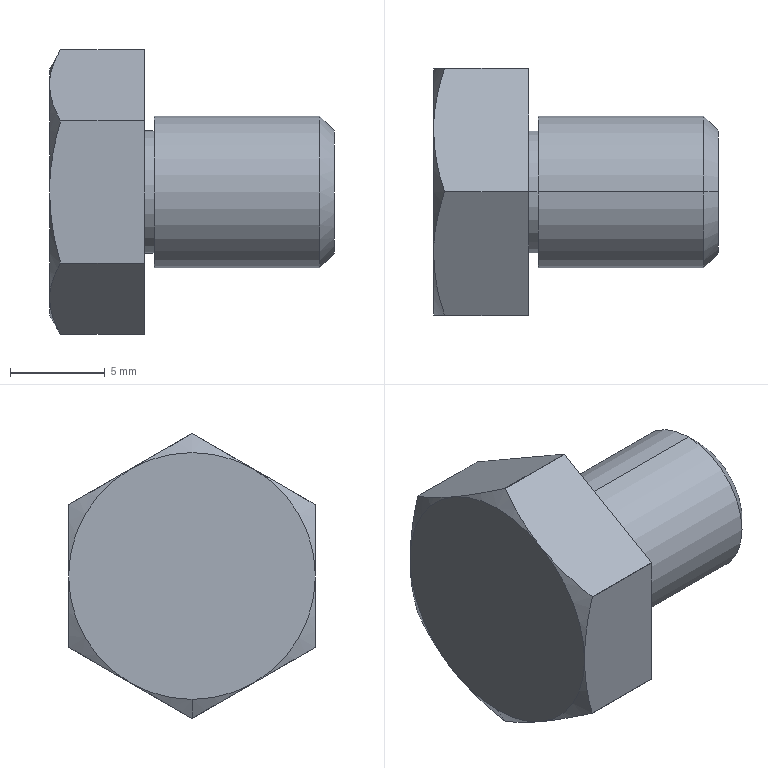Part | STEP file | SSTEH13-4 | 1 solid | 30 faces | box 15 x 13 x 15 mm | volume 1216 mm3 | cylinder 11 | plane 10 | cone 9 | commonest cylinder face diameters 15 x7 6.466 x2 8 x2
STEP:
#1=CARTESIAN_POINT('',(10.,0.,3.233));
#2=VERTEX_POINT('',#1);
#3=CARTESIAN_POINT('',(10.,0.,-3.233));
#4=VERTEX_POINT('',#3);
#5=CARTESIAN_POINT('',(10.,0.,0.));
#6=DIRECTION('',(-1.,0.,0.));
#7=DIRECTION('',(0.,0.,-1.));
#8=AXIS2_PLACEMENT_3D('',#5,#6,#7);
#9=CIRCLE('',#8,3.233);
#10=EDGE_CURVE('',#2,#4,#9,.T.);
#11=ORIENTED_EDGE('',*,*,#10,.T.);
#12=CARTESIAN_POINT('',(9.233,0.,-4.));
#13=VERTEX_POINT('',#12);
#14=CARTESIAN_POINT('',(9.233,0.,-4.));
#15=DIRECTION('',(-0.7071,0.,-0.7071));
#16=VECTOR('',#15,1000.);
#17=LINE('',#14,#16);
#18=EDGE_CURVE('',#4,#13,#17,.T.);
#19=ORIENTED_EDGE('',*,*,#18,.T.);
#20=CARTESIAN_POINT('',(9.233,0.,4.));
#21=VERTEX_POINT('',#20);
#22=CARTESIAN_POINT('',(9.233,0.,0.));
#23=DIRECTION('',(-1.,0.,0.));
#24=DIRECTION('',(0.,0.,-1.));
#25=AXIS2_PLACEMENT_3D('',#22,#23,#24);
#26=CIRCLE('',#25,4.);
#27=EDGE_CURVE('',#21,#13,#26,.T.);
#28=ORIENTED_EDGE('',*,*,#27,.F.);
#29=CARTESIAN_POINT('',(9.233,0.,4.));
#30=DIRECTION('',(-0.7071,0.,0.7071));
#31=VECTOR('',#30,1000.);
#32=LINE('',#29,#31);
#33=EDGE_CURVE('',#2,#21,#32,.T.);
#34=ORIENTED_EDGE('',*,*,#33,.F.);
#35=EDGE_LOOP('',(#11,#19,#28,#34));
#36=FACE_OUTER_BOUND('',#35,.T.);
#37=CARTESIAN_POINT('',(9.233,0.,0.));
#38=DIRECTION('',(-1.,0.,0.));
#39=DIRECTION('',(0.,0.,1.));
#40=AXIS2_PLACEMENT_3D('',#37,#38,#39);
#41=CONICAL_SURFACE('',#40,4.,0.7854);
#42=ADVANCED_FACE('',(#36),#41,.T.);
#43=CARTESIAN_POINT('',(0.5,0.,4.));
#44=VERTEX_POINT('',#43);
#45=CARTESIAN_POINT('',(0.5,0.,-4.));
#46=VERTEX_POINT('',#45);
#47=CARTESIAN_POINT('',(0.5,0.,0.));
#48=DIRECTION('',(-1.,0.,0.));
#49=DIRECTION('',(0.,0.,-1.));
#50=AXIS2_PLACEMENT_3D('',#47,#48,#49);
#51=CIRCLE('',#50,4.);
#52=EDGE_CURVE('',#44,#46,#51,.T.);
#53=ORIENTED_EDGE('',*,*,#52,.F.);
#54=CARTESIAN_POINT('',(10.,0.,4.));
#55=DIRECTION('',(1.,0.,0.));
#56=VECTOR('',#55,1000.);
#57=LINE('',#54,#56);
#58=EDGE_CURVE('',#44,#21,#57,.T.);
#59=ORIENTED_EDGE('',*,*,#58,.T.);
#60=ORIENTED_EDGE('',*,*,#27,.T.);
#61=CARTESIAN_POINT('',(10.,0.,-4.));
#62=DIRECTION('',(1.,0.,0.));
#63=VECTOR('',#62,1000.);
#64=LINE('',#61,#63);
#65=EDGE_CURVE('',#46,#13,#64,.T.);
#66=ORIENTED_EDGE('',*,*,#65,.F.);
#67=EDGE_LOOP('',(#53,#59,#60,#66));
#68=FACE_OUTER_BOUND('',#67,.T.);
#69=CARTESIAN_POINT('',(10.,0.,0.));
#70=DIRECTION('',(1.,0.,0.));
#71=DIRECTION('',(0.,0.,-1.));
#72=AXIS2_PLACEMENT_3D('',#69,#70,#71);
#73=CYLINDRICAL_SURFACE('',#72,4.);
#74=ADVANCED_FACE('',(#68),#73,.T.);
#75=CARTESIAN_POINT('',(0.,0.,3.233));
#76=VERTEX_POINT('',#75);
#77=CARTESIAN_POINT('',(0.,0.,-3.233));
#78=VERTEX_POINT('',#77);
#79=CARTESIAN_POINT('',(0.,0.,0.));
#80=DIRECTION('',(-1.,0.,0.));
#81=DIRECTION('',(0.,0.,-1.));
#82=AXIS2_PLACEMENT_3D('',#79,#80,#81);
#83=CIRCLE('',#82,3.233);
#84=EDGE_CURVE('',#76,#78,#83,.T.);
#85=ORIENTED_EDGE('',*,*,#84,.F.);
#86=CARTESIAN_POINT('',(0.5,0.,3.233));
#87=VERTEX_POINT('',#86);
#88=CARTESIAN_POINT('',(10.,0.,3.233));
#89=DIRECTION('',(1.,0.,0.));
#90=VECTOR('',#89,1000.);
#91=LINE('',#88,#90);
#92=EDGE_CURVE('',#76,#87,#91,.T.);
#93=ORIENTED_EDGE('',*,*,#92,.T.);
#94=CARTESIAN_POINT('',(0.5,0.,-3.233));
#95=VERTEX_POINT('',#94);
#96=CARTESIAN_POINT('',(0.5,0.,0.));
#97=DIRECTION('',(-1.,0.,0.));
#98=DIRECTION('',(0.,0.,-1.));
#99=AXIS2_PLACEMENT_3D('',#96,#97,#98);
#100=CIRCLE('',#99,3.233);
#101=EDGE_CURVE('',#87,#95,#100,.T.);
#102=ORIENTED_EDGE('',*,*,#101,.T.);
#103=CARTESIAN_POINT('',(10.,0.,-3.233));
#104=DIRECTION('',(1.,0.,0.));
#105=VECTOR('',#104,1000.);
#106=LINE('',#103,#105);
#107=EDGE_CURVE('',#78,#95,#106,.T.);
#108=ORIENTED_EDGE('',*,*,#107,.F.);
#109=EDGE_LOOP('',(#85,#93,#102,#108));
#110=FACE_OUTER_BOUND('',#109,.T.);
#111=CARTESIAN_POINT('',(10.,0.,0.));
#112=DIRECTION('',(1.,0.,0.));
#113=DIRECTION('',(0.,0.,-1.));
#114=AXIS2_PLACEMENT_3D('',#111,#112,#113);
#115=CYLINDRICAL_SURFACE('',#114,3.233);
#116=ADVANCED_FACE('',(#110),#115,.T.);
#117=CARTESIAN_POINT('',(-4.423,0.,-7.5));
#118=VERTEX_POINT('',#117);
#119=CARTESIAN_POINT('',(-4.423,-0.00963,-7.5));
#120=VERTEX_POINT('',#119);
#121=CARTESIAN_POINT('',(-4.423,0.,0.));
#122=DIRECTION('',(-1.,0.,0.));
#123=DIRECTION('',(0.,0.,-1.));
#124=AXIS2_PLACEMENT_3D('',#121,#122,#123);
#125=CIRCLE('',#124,7.5);
#126=EDGE_CURVE('',#118,#120,#125,.T.);
#127=ORIENTED_EDGE('',*,*,#126,.F.);
#128=CARTESIAN_POINT('',(0.,0.,-7.5));
#129=VERTEX_POINT('',#128);
#130=CARTESIAN_POINT('',(10.,0.,-7.5));
#131=DIRECTION('',(1.,0.,0.));
#132=VECTOR('',#131,1000.);
#133=LINE('',#130,#132);
#134=EDGE_CURVE('',#118,#129,#133,.T.);
#135=ORIENTED_EDGE('',*,*,#134,.T.);
#136=CARTESIAN_POINT('',(0.,-0.00963,-7.5));
#137=VERTEX_POINT('',#136);
#138=CARTESIAN_POINT('',(0.,0.,0.));
#139=DIRECTION('',(-1.,0.,0.));
#140=DIRECTION('',(0.,0.,-1.));
#141=AXIS2_PLACEMENT_3D('',#138,#139,#140);
#142=CIRCLE('',#141,7.5);
#143=EDGE_CURVE('',#129,#137,#142,.T.);
#144=ORIENTED_EDGE('',*,*,#143,.T.);
#145=CARTESIAN_POINT('',(10.,-0.00963,-7.5));
#146=DIRECTION('',(-1.,0.,0.));
#147=VECTOR('',#146,1000.);
#148=LINE('',#145,#147);
#149=EDGE_CURVE('',#137,#120,#148,.T.);
#150=ORIENTED_EDGE('',*,*,#149,.T.);
#151=EDGE_LOOP('',(#127,#135,#144,#150));
#152=FACE_OUTER_BOUND('',#151,.T.);
#153=CARTESIAN_POINT('',(10.,0.,0.));
#154=DIRECTION('',(1.,0.,0.));
#155=DIRECTION('',(0.,0.,-1.));
#156=AXIS2_PLACEMENT_3D('',#153,#154,#155);
#157=CYLINDRICAL_SURFACE('',#156,7.5);
#158=ADVANCED_FACE('',(#152),#157,.T.);
#159=CARTESIAN_POINT('',(-5.,0.,-6.5));
#160=VERTEX_POINT('',#159);
#161=CARTESIAN_POINT('',(-5.,-3.25,-5.629));
#162=VERTEX_POINT('',#161);
#163=CARTESIAN_POINT('',(-5.,0.,0.));
#164=DIRECTION('',(-1.,0.,0.));
#165=DIRECTION('',(0.,0.,-1.));
#166=AXIS2_PLACEMENT_3D('',#163,#164,#165);
#167=CIRCLE('',#166,6.5);
#168=EDGE_CURVE('',#160,#162,#167,.T.);
#169=ORIENTED_EDGE('',*,*,#168,.F.);
#170=CARTESIAN_POINT('',(-5.,0.,-6.5));
#171=DIRECTION('',(0.5,0.,-0.866));
#172=VECTOR('',#171,1000.);
#173=LINE('',#170,#172);
#174=EDGE_CURVE('',#160,#118,#173,.T.);
#175=ORIENTED_EDGE('',*,*,#174,.T.);
#176=ORIENTED_EDGE('',*,*,#126,.T.);
#177=CARTESIAN_POINT('',(-4.423,-0.00963,-7.5));
#178=CARTESIAN_POINT('',(-4.599,-0.5398,-7.194));
#179=CARTESIAN_POINT('',(-4.744,-1.074,-6.886));
#180=CARTESIAN_POINT('',(-4.945,-2.153,-6.263));
#181=CARTESIAN_POINT('',(-5.,-2.698,-5.948));
#182=CARTESIAN_POINT('',(-5.,-3.25,-5.629));
#183=B_SPLINE_CURVE_WITH_KNOTS('',3,(#177,#178,#179,#180,#181,#182),.UNSPECIFIED.,.F.,.F.,(4,2,4),(0.000000425,0.001893,0.003786),.UNSPECIFIED.);
#184=EDGE_CURVE('',#120,#162,#183,.T.);
#185=ORIENTED_EDGE('',*,*,#184,.T.);
#186=EDGE_LOOP('',(#169,#175,#176,#185));
#187=FACE_OUTER_BOUND('',#186,.T.);
#188=CARTESIAN_POINT('',(-5.,0.,0.));
#189=DIRECTION('',(1.,0.,0.));
#190=DIRECTION('',(0.,0.,-1.));
#191=AXIS2_PLACEMENT_3D('',#188,#189,#190);
#192=CONICAL_SURFACE('',#191,6.5,1.047);
#193=ADVANCED_FACE('',(#187),#192,.T.);
#194=CARTESIAN_POINT('',(-4.423,6.5,3.742));
#195=VERTEX_POINT('',#194);
#196=CARTESIAN_POINT('',(-5.,6.5,0.));
#197=VERTEX_POINT('',#196);
#198=CARTESIAN_POINT('',(-4.423,6.5,3.742));
#199=CARTESIAN_POINT('',(-4.774,6.5,2.523));
#200=CARTESIAN_POINT('',(-5.,6.5,1.281));
#201=CARTESIAN_POINT('',(-5.,6.5,0.));
#202=B_SPLINE_CURVE_WITH_KNOTS('',3,(#198,#199,#200,#201),.UNSPECIFIED.,.F.,.F.,(4,4),(0.008188,0.01199),.UNSPECIFIED.);
#203=EDGE_CURVE('',#195,#197,#202,.T.);
#204=ORIENTED_EDGE('',*,*,#203,.T.);
#205=CARTESIAN_POINT('',(-5.,3.25,5.629));
#206=VERTEX_POINT('',#205);
#207=CARTESIAN_POINT('',(-5.,0.,0.));
#208=DIRECTION('',(-1.,0.,0.));
#209=DIRECTION('',(0.,0.,-1.));
#210=AXIS2_PLACEMENT_3D('',#207,#208,#209);
#211=CIRCLE('',#210,6.5);
#212=EDGE_CURVE('',#206,#197,#211,.T.);
#213=ORIENTED_EDGE('',*,*,#212,.F.);
#214=CARTESIAN_POINT('',(-4.423,6.49,3.758));
#215=VERTEX_POINT('',#214);
#216=CARTESIAN_POINT('',(-5.,3.25,5.629));
#217=CARTESIAN_POINT('',(-5.,3.525,5.47));
#218=CARTESIAN_POINT('',(-4.986,3.801,5.311));
#219=CARTESIAN_POINT('',(-4.934,4.348,4.995));
#220=CARTESIAN_POINT('',(-4.894,4.619,4.839));
#221=CARTESIAN_POINT('',(-4.744,5.428,4.371));
#222=CARTESIAN_POINT('',(-4.599,5.962,4.064));
#223=CARTESIAN_POINT('',(-4.423,6.49,3.758));
#224=B_SPLINE_CURVE_WITH_KNOTS('',3,(#216,#217,#218,#219,#220,#221,#222,#223),.UNSPECIFIED.,.F.,.F.,(4,2,2,4),(0.003786,0.004729,0.005672,0.007557),.UNSPECIFIED.);
#225=EDGE_CURVE('',#206,#215,#224,.T.);
#226=ORIENTED_EDGE('',*,*,#225,.T.);
#227=CARTESIAN_POINT('',(-4.423,0.,0.));
#228=DIRECTION('',(-1.,0.,0.));
#229=DIRECTION('',(0.,0.,-1.));
#230=AXIS2_PLACEMENT_3D('',#227,#228,#229);
#231=CIRCLE('',#230,7.5);
#232=EDGE_CURVE('',#215,#195,#231,.T.);
#233=ORIENTED_EDGE('',*,*,#232,.T.);
#234=EDGE_LOOP('',(#204,#213,#226,#233));
#235=FACE_OUTER_BOUND('',#234,.T.);
#236=CARTESIAN_POINT('',(-5.,0.,0.));
#237=DIRECTION('',(1.,0.,0.));
#238=DIRECTION('',(0.,0.,-1.));
#239=AXIS2_PLACEMENT_3D('',#236,#237,#238);
#240=CONICAL_SURFACE('',#239,6.5,1.047);
#241=ADVANCED_FACE('',(#235),#240,.T.);
#242=CARTESIAN_POINT('',(-4.423,6.5,-3.742));
#243=VERTEX_POINT('',#242);
#244=CARTESIAN_POINT('',(-5.,6.5,0.));
#245=CARTESIAN_POINT('',(-5.,6.5,-0.6403));
#246=CARTESIAN_POINT('',(-4.944,6.5,-1.273));
#247=CARTESIAN_POINT('',(-4.743,6.5,-2.518));
#248=CARTESIAN_POINT('',(-4.598,6.5,-3.133));
#249=CARTESIAN_POINT('',(-4.423,6.5,-3.742));
#250=B_SPLINE_CURVE_WITH_KNOTS('',3,(#244,#245,#246,#247,#248,#249),.UNSPECIFIED.,.F.,.F.,(4,2,4),(0.01199,0.0139,0.0158),.UNSPECIFIED.);
#251=EDGE_CURVE('',#197,#243,#250,.T.);
#252=ORIENTED_EDGE('',*,*,#251,.T.);
#253=CARTESIAN_POINT('',(-4.423,6.49,-3.758));
#254=VERTEX_POINT('',#253);
#255=CARTESIAN_POINT('',(-4.423,0.,0.));
#256=DIRECTION('',(-1.,0.,0.));
#257=DIRECTION('',(0.,0.,-1.));
#258=AXIS2_PLACEMENT_3D('',#255,#256,#257);
#259=CIRCLE('',#258,7.5);
#260=EDGE_CURVE('',#243,#254,#259,.T.);
#261=ORIENTED_EDGE('',*,*,#260,.T.);
#262=CARTESIAN_POINT('',(-5.,3.25,-5.629));
#263=VERTEX_POINT('',#262);
#264=CARTESIAN_POINT('',(-4.423,6.49,-3.758));
#265=CARTESIAN_POINT('',(-4.599,5.96,-4.064));
#266=CARTESIAN_POINT('',(-4.744,5.426,-4.373));
#267=CARTESIAN_POINT('',(-4.945,4.347,-4.996));
#268=CARTESIAN_POINT('',(-5.,3.802,-5.31));
#269=CARTESIAN_POINT('',(-5.,3.25,-5.629));
#270=B_SPLINE_CURVE_WITH_KNOTS('',3,(#264,#265,#266,#267,#268,#269),.UNSPECIFIED.,.F.,.F.,(4,2,4),(0.000000716,0.001894,0.003786),.UNSPECIFIED.);
#271=EDGE_CURVE('',#254,#263,#270,.T.);
#272=ORIENTED_EDGE('',*,*,#271,.T.);
#273=CARTESIAN_POINT('',(-5.,0.,0.));
#274=DIRECTION('',(-1.,0.,0.));
#275=DIRECTION('',(0.,0.,-1.));
#276=AXIS2_PLACEMENT_3D('',#273,#274,#275);
#277=CIRCLE('',#276,6.5);
#278=EDGE_CURVE('',#197,#263,#277,.T.);
#279=ORIENTED_EDGE('',*,*,#278,.F.);
#280=EDGE_LOOP('',(#252,#261,#272,#279));
#281=FACE_OUTER_BOUND('',#280,.T.);
#282=CARTESIAN_POINT('',(-5.,0.,0.));
#283=DIRECTION('',(1.,0.,0.));
#284=DIRECTION('',(0.,0.,-1.));
#285=AXIS2_PLACEMENT_3D('',#282,#283,#284);
#286=CONICAL_SURFACE('',#285,6.5,1.047);
#287=ADVANCED_FACE('',(#281),#286,.T.);
#288=ORIENTED_EDGE('',*,*,#174,.F.);
#289=CARTESIAN_POINT('',(-5.,0.,0.));
#290=DIRECTION('',(-1.,0.,0.));
#291=DIRECTION('',(0.,0.,-1.));
#292=AXIS2_PLACEMENT_3D('',#289,#290,#291);
#293=CIRCLE('',#292,6.5);
#294=EDGE_CURVE('',#263,#160,#293,.T.);
#295=ORIENTED_EDGE('',*,*,#294,.F.);
#296=CARTESIAN_POINT('',(-4.423,0.00963,-7.5));
#297=VERTEX_POINT('',#296);
#298=CARTESIAN_POINT('',(-5.,3.25,-5.629));
#299=CARTESIAN_POINT('',(-5.,2.975,-5.788));
#300=CARTESIAN_POINT('',(-4.986,2.699,-5.947));
#301=CARTESIAN_POINT('',(-4.934,2.152,-6.263));
#302=CARTESIAN_POINT('',(-4.894,1.881,-6.42));
#303=CARTESIAN_POINT('',(-4.744,1.072,-6.887));
#304=CARTESIAN_POINT('',(-4.599,0.5384,-7.195));
#305=CARTESIAN_POINT('',(-4.423,0.00963,-7.5));
#306=B_SPLINE_CURVE_WITH_KNOTS('',3,(#298,#299,#300,#301,#302,#303,#304,#305),.UNSPECIFIED.,.F.,.F.,(4,2,2,4),(0.003786,0.004729,0.005672,0.007558),.UNSPECIFIED.);
#307=EDGE_CURVE('',#263,#297,#306,.T.);
#308=ORIENTED_EDGE('',*,*,#307,.T.);
#309=CARTESIAN_POINT('',(-4.423,0.,0.));
#310=DIRECTION('',(-1.,0.,0.));
#311=DIRECTION('',(0.,0.,-1.));
#312=AXIS2_PLACEMENT_3D('',#309,#310,#311);
#313=CIRCLE('',#312,7.5);
#314=EDGE_CURVE('',#297,#118,#313,.T.);
#315=ORIENTED_EDGE('',*,*,#314,.T.);
#316=EDGE_LOOP('',(#288,#295,#308,#315));
#317=FACE_OUTER_BOUND('',#316,.T.);
#318=CARTESIAN_POINT('',(-5.,0.,0.));
#319=DIRECTION('',(1.,0.,0.));
#320=DIRECTION('',(0.,0.,-1.));
#321=AXIS2_PLACEMENT_3D('',#318,#319,#320);
#322=CONICAL_SURFACE('',#321,6.5,1.047);
#323=ADVANCED_FACE('',(#317),#322,.T.);
#324=CARTESIAN_POINT('',(-4.423,-6.49,-3.758));
#325=VERTEX_POINT('',#324);
#326=CARTESIAN_POINT('',(-5.,-3.25,-5.629));
#327=CARTESIAN_POINT('',(-5.,-3.525,-5.47));
#328=CARTESIAN_POINT('',(-4.986,-3.801,-5.311));
#329=CARTESIAN_POINT('',(-4.934,-4.348,-4.995));
#330=CARTESIAN_POINT('',(-4.894,-4.619,-4.839));
#331=CARTESIAN_POINT('',(-4.744,-5.428,-4.371));
#332=CARTESIAN_POINT('',(-4.599,-5.962,-4.064));
#333=CARTESIAN_POINT('',(-4.423,-6.49,-3.758));
#334=B_SPLINE_CURVE_WITH_KNOTS('',3,(#326,#327,#328,#329,#330,#331,#332,#333),.UNSPECIFIED.,.F.,.F.,(4,2,2,4),(0.003786,0.004729,0.005672,0.007557),.UNSPECIFIED.);
#335=EDGE_CURVE('',#162,#325,#334,.T.);
#336=ORIENTED_EDGE('',*,*,#335,.T.);
#337=CARTESIAN_POINT('',(-4.423,-6.5,-3.742));
#338=VERTEX_POINT('',#337);
#339=CARTESIAN_POINT('',(-4.423,0.,0.));
#340=DIRECTION('',(-1.,0.,0.));
#341=DIRECTION('',(0.,0.,-1.));
#342=AXIS2_PLACEMENT_3D('',#339,#340,#341);
#343=CIRCLE('',#342,7.5);
#344=EDGE_CURVE('',#325,#338,#343,.T.);
#345=ORIENTED_EDGE('',*,*,#344,.T.);
#346=CARTESIAN_POINT('',(-5.,-6.5,0.));
#347=VERTEX_POINT('',#346);
#348=CARTESIAN_POINT('',(-4.423,-6.5,-3.742));
#349=CARTESIAN_POINT('',(-4.774,-6.5,-2.523));
#350=CARTESIAN_POINT('',(-5.,-6.5,-1.281));
#351=CARTESIAN_POINT('',(-5.,-6.5,0.));
#352=B_SPLINE_CURVE_WITH_KNOTS('',3,(#348,#349,#350,#351),.UNSPECIFIED.,.F.,.F.,(4,4),(0.008188,0.01199),.UNSPECIFIED.);
#353=EDGE_CURVE('',#338,#347,#352,.T.);
#354=ORIENTED_EDGE('',*,*,#353,.T.);
#355=CARTESIAN_POINT('',(-5.,0.,0.));
#356=DIRECTION('',(-1.,0.,0.));
#357=DIRECTION('',(0.,0.,-1.));
#358=AXIS2_PLACEMENT_3D('',#355,#356,#357);
#359=CIRCLE('',#358,6.5);
#360=EDGE_CURVE('',#162,#347,#359,.T.);
#361=ORIENTED_EDGE('',*,*,#360,.F.);
#362=EDGE_LOOP('',(#336,#345,#354,#361));
#363=FACE_OUTER_BOUND('',#362,.T.);
#364=CARTESIAN_POINT('',(-5.,0.,0.));
#365=DIRECTION('',(1.,0.,0.));
#366=DIRECTION('',(0.,0.,-1.));
#367=AXIS2_PLACEMENT_3D('',#364,#365,#366);
#368=CONICAL_SURFACE('',#367,6.5,1.047);
#369=ADVANCED_FACE('',(#363),#368,.T.);
#370=CARTESIAN_POINT('',(-4.423,-6.5,3.742));
#371=VERTEX_POINT('',#370);
#372=CARTESIAN_POINT('',(-5.,-6.5,0.));
#373=CARTESIAN_POINT('',(-5.,-6.5,0.6403));
#374=CARTESIAN_POINT('',(-4.944,-6.5,1.273));
#375=CARTESIAN_POINT('',(-4.743,-6.5,2.518));
#376=CARTESIAN_POINT('',(-4.598,-6.5,3.133));
#377=CARTESIAN_POINT('',(-4.423,-6.5,3.742));
#378=B_SPLINE_CURVE_WITH_KNOTS('',3,(#372,#373,#374,#375,#376,#377),.UNSPECIFIED.,.F.,.F.,(4,2,4),(0.01199,0.0139,0.0158),.UNSPECIFIED.);
#379=EDGE_CURVE('',#347,#371,#378,.T.);
#380=ORIENTED_EDGE('',*,*,#379,.T.);
#381=CARTESIAN_POINT('',(-4.423,-6.49,3.758));
#382=VERTEX_POINT('',#381);
#383=CARTESIAN_POINT('',(-4.423,0.,0.));
#384=DIRECTION('',(-1.,0.,0.));
#385=DIRECTION('',(0.,0.,-1.));
#386=AXIS2_PLACEMENT_3D('',#383,#384,#385);
#387=CIRCLE('',#386,7.5);
#388=EDGE_CURVE('',#371,#382,#387,.T.);
#389=ORIENTED_EDGE('',*,*,#388,.T.);
#390=CARTESIAN_POINT('',(-5.,-3.25,5.629));
#391=VERTEX_POINT('',#390);
#392=CARTESIAN_POINT('',(-4.423,-6.49,3.758));
#393=CARTESIAN_POINT('',(-4.599,-5.96,4.064));
#394=CARTESIAN_POINT('',(-4.744,-5.426,4.373));
#395=CARTESIAN_POINT('',(-4.945,-4.347,4.996));
#396=CARTESIAN_POINT('',(-5.,-3.802,5.31));
#397=CARTESIAN_POINT('',(-5.,-3.25,5.629));
#398=B_SPLINE_CURVE_WITH_KNOTS('',3,(#392,#393,#394,#395,#396,#397),.UNSPECIFIED.,.F.,.F.,(4,2,4),(0.000000716,0.001894,0.003786),.UNSPECIFIED.);
#399=EDGE_CURVE('',#382,#391,#398,.T.);
#400=ORIENTED_EDGE('',*,*,#399,.T.);
#401=CARTESIAN_POINT('',(-5.,0.,0.));
#402=DIRECTION('',(-1.,0.,0.));
#403=DIRECTION('',(0.,0.,-1.));
#404=AXIS2_PLACEMENT_3D('',#401,#402,#403);
#405=CIRCLE('',#404,6.5);
#406=EDGE_CURVE('',#347,#391,#405,.T.);
#407=ORIENTED_EDGE('',*,*,#406,.F.);
#408=EDGE_LOOP('',(#380,#389,#400,#407));
#409=FACE_OUTER_BOUND('',#408,.T.);
#410=CARTESIAN_POINT('',(-5.,0.,0.));
#411=DIRECTION('',(1.,0.,0.));
#412=DIRECTION('',(0.,0.,-1.));
#413=AXIS2_PLACEMENT_3D('',#410,#411,#412);
#414=CONICAL_SURFACE('',#413,6.5,1.047);
#415=ADVANCED_FACE('',(#409),#414,.T.);
#416=CARTESIAN_POINT('',(-4.423,-0.00963,7.5));
#417=VERTEX_POINT('',#416);
#418=CARTESIAN_POINT('',(-5.,-3.25,5.629));
#419=CARTESIAN_POINT('',(-5.,-2.975,5.788));
#420=CARTESIAN_POINT('',(-4.986,-2.699,5.947));
#421=CARTESIAN_POINT('',(-4.934,-2.152,6.263));
#422=CARTESIAN_POINT('',(-4.894,-1.881,6.42));
#423=CARTESIAN_POINT('',(-4.744,-1.072,6.887));
#424=CARTESIAN_POINT('',(-4.599,-0.5384,7.195));
#425=CARTESIAN_POINT('',(-4.423,-0.00963,7.5));
#426=B_SPLINE_CURVE_WITH_KNOTS('',3,(#418,#419,#420,#421,#422,#423,#424,#425),.UNSPECIFIED.,.F.,.F.,(4,2,2,4),(0.003786,0.004729,0.005672,0.007558),.UNSPECIFIED.);
#427=EDGE_CURVE('',#391,#417,#426,.T.);
#428=ORIENTED_EDGE('',*,*,#427,.T.);
#429=CARTESIAN_POINT('',(-4.423,0.00963,7.5));
#430=VERTEX_POINT('',#429);
#431=CARTESIAN_POINT('',(-4.423,0.,0.));
#432=DIRECTION('',(-1.,0.,0.));
#433=DIRECTION('',(0.,0.,-1.));
#434=AXIS2_PLACEMENT_3D('',#431,#432,#433);
#435=CIRCLE('',#434,7.5);
#436=EDGE_CURVE('',#417,#430,#435,.T.);
#437=ORIENTED_EDGE('',*,*,#436,.T.);
#438=CARTESIAN_POINT('',(-4.423,0.00963,7.5));
#439=CARTESIAN_POINT('',(-4.599,0.5398,7.194));
#440=CARTESIAN_POINT('',(-4.744,1.074,6.886));
#441=CARTESIAN_POINT('',(-4.945,2.153,6.263));
#442=CARTESIAN_POINT('',(-5.,2.698,5.948));
#443=CARTESIAN_POINT('',(-5.,3.25,5.629));
#444=B_SPLINE_CURVE_WITH_KNOTS('',3,(#438,#439,#440,#441,#442,#443),.UNSPECIFIED.,.F.,.F.,(4,2,4),(0.000000425,0.001893,0.003786),.UNSPECIFIED.);
#445=EDGE_CURVE('',#430,#206,#444,.T.);
#446=ORIENTED_EDGE('',*,*,#445,.T.);
#447=CARTESIAN_POINT('',(-5.,0.,0.));
#448=DIRECTION('',(-1.,0.,0.));
#449=DIRECTION('',(0.,0.,-1.));
#450=AXIS2_PLACEMENT_3D('',#447,#448,#449);
#451=CIRCLE('',#450,6.5);
#452=EDGE_CURVE('',#391,#206,#451,.T.);
#453=ORIENTED_EDGE('',*,*,#452,.F.);
#454=EDGE_LOOP('',(#428,#437,#446,#453));
#455=FACE_OUTER_BOUND('',#454,.T.);
#456=CARTESIAN_POINT('',(-5.,0.,0.));
#457=DIRECTION('',(1.,0.,0.));
#458=DIRECTION('',(0.,0.,-1.));
#459=AXIS2_PLACEMENT_3D('',#456,#457,#458);
#460=CONICAL_SURFACE('',#459,6.5,1.047);
#461=ADVANCED_FACE('',(#455),#460,.T.);
#462=CARTESIAN_POINT('',(0.,6.5,-3.742));
#463=VERTEX_POINT('',#462);
#464=CARTESIAN_POINT('',(10.,6.5,-3.742));
#465=DIRECTION('',(1.,0.,0.));
#466=VECTOR('',#465,1000.);
#467=LINE('',#464,#466);
#468=EDGE_CURVE('',#243,#463,#467,.T.);
#469=ORIENTED_EDGE('',*,*,#468,.T.);
#470=CARTESIAN_POINT('',(0.,6.49,-3.758));
#471=VERTEX_POINT('',#470);
#472=CARTESIAN_POINT('',(0.,0.,0.));
#473=DIRECTION('',(-1.,0.,0.));
#474=DIRECTION('',(0.,0.,-1.));
#475=AXIS2_PLACEMENT_3D('',#472,#473,#474);
#476=CIRCLE('',#475,7.5);
#477=EDGE_CURVE('',#463,#471,#476,.T.);
#478=ORIENTED_EDGE('',*,*,#477,.T.);
#479=CARTESIAN_POINT('',(10.,6.49,-3.758));
#480=DIRECTION('',(-1.,0.,0.));
#481=VECTOR('',#480,1000.);
#482=LINE('',#479,#481);
#483=EDGE_CURVE('',#471,#254,#482,.T.);
#484=ORIENTED_EDGE('',*,*,#483,.T.);
#485=ORIENTED_EDGE('',*,*,#260,.F.);
#486=EDGE_LOOP('',(#469,#478,#484,#485));
#487=FACE_OUTER_BOUND('',#486,.T.);
#488=CARTESIAN_POINT('',(10.,0.,0.));
#489=DIRECTION('',(1.,0.,0.));
#490=DIRECTION('',(0.,0.,-1.));
#491=AXIS2_PLACEMENT_3D('',#488,#489,#490);
#492=CYLINDRICAL_SURFACE('',#491,7.5);
#493=ADVANCED_FACE('',(#487),#492,.T.);
#494=CARTESIAN_POINT('',(0.,6.5,3.742));
#495=VERTEX_POINT('',#494);
#496=CARTESIAN_POINT('',(10.,6.5,3.742));
#497=DIRECTION('',(-1.,0.,0.));
#498=VECTOR('',#497,1000.);
#499=LINE('',#496,#498);
#500=EDGE_CURVE('',#495,#195,#499,.T.);
#501=ORIENTED_EDGE('',*,*,#500,.T.);
#502=ORIENTED_EDGE('',*,*,#232,.F.);
#503=CARTESIAN_POINT('',(0.,6.49,3.758));
#504=VERTEX_POINT('',#503);
#505=CARTESIAN_POINT('',(10.,6.49,3.758));
#506=DIRECTION('',(1.,0.,0.));
#507=VECTOR('',#506,1000.);
#508=LINE('',#505,#507);
#509=EDGE_CURVE('',#215,#504,#508,.T.);
#510=ORIENTED_EDGE('',*,*,#509,.T.);
#511=CARTESIAN_POINT('',(0.,0.,0.));
#512=DIRECTION('',(-1.,0.,0.));
#513=DIRECTION('',(0.,0.,-1.));
#514=AXIS2_PLACEMENT_3D('',#511,#512,#513);
#515=CIRCLE('',#514,7.5);
#516=EDGE_CURVE('',#504,#495,#515,.T.);
#517=ORIENTED_EDGE('',*,*,#516,.T.);
#518=EDGE_LOOP('',(#501,#502,#510,#517));
#519=FACE_OUTER_BOUND('',#518,.T.);
#520=CARTESIAN_POINT('',(10.,0.,0.));
#521=DIRECTION('',(1.,0.,0.));
#522=DIRECTION('',(0.,0.,-1.));
#523=AXIS2_PLACEMENT_3D('',#520,#521,#522);
#524=CYLINDRICAL_SURFACE('',#523,7.5);
#525=ADVANCED_FACE('',(#519),#524,.T.);
#526=ORIENTED_EDGE('',*,*,#134,.F.);
#527=ORIENTED_EDGE('',*,*,#314,.F.);
#528=CARTESIAN_POINT('',(0.,0.00963,-7.5));
#529=VERTEX_POINT('',#528);
#530=CARTESIAN_POINT('',(10.,0.00963,-7.5));
#531=DIRECTION('',(1.,0.,0.));
#532=VECTOR('',#531,1000.);
#533=LINE('',#530,#532);
#534=EDGE_CURVE('',#297,#529,#533,.T.);
#535=ORIENTED_EDGE('',*,*,#534,.T.);
#536=CARTESIAN_POINT('',(0.,0.,0.));
#537=DIRECTION('',(-1.,0.,0.));
#538=DIRECTION('',(0.,0.,-1.));
#539=AXIS2_PLACEMENT_3D('',#536,#537,#538);
#540=CIRCLE('',#539,7.5);
#541=EDGE_CURVE('',#529,#129,#540,.T.);
#542=ORIENTED_EDGE('',*,*,#541,.T.);
#543=EDGE_LOOP('',(#526,#527,#535,#542));
#544=FACE_OUTER_BOUND('',#543,.T.);
#545=CARTESIAN_POINT('',(10.,0.,0.));
#546=DIRECTION('',(1.,0.,0.));
#547=DIRECTION('',(0.,0.,-1.));
#548=AXIS2_PLACEMENT_3D('',#545,#546,#547);
#549=CYLINDRICAL_SURFACE('',#548,7.5);
#550=ADVANCED_FACE('',(#544),#549,.T.);
#551=CARTESIAN_POINT('',(0.,-6.49,-3.758));
#552=VERTEX_POINT('',#551);
#553=CARTESIAN_POINT('',(10.,-6.49,-3.758));
#554=DIRECTION('',(1.,0.,0.));
#555=VECTOR('',#554,1000.);
#556=LINE('',#553,#555);
#557=EDGE_CURVE('',#325,#552,#556,.T.);
#558=ORIENTED_EDGE('',*,*,#557,.T.);
#559=CARTESIAN_POINT('',(0.,-6.5,-3.742));
#560=VERTEX_POINT('',#559);
#561=CARTESIAN_POINT('',(0.,0.,0.));
#562=DIRECTION('',(-1.,0.,0.));
#563=DIRECTION('',(0.,0.,-1.));
#564=AXIS2_PLACEMENT_3D('',#561,#562,#563);
#565=CIRCLE('',#564,7.5);
#566=EDGE_CURVE('',#552,#560,#565,.T.);
#567=ORIENTED_EDGE('',*,*,#566,.T.);
#568=CARTESIAN_POINT('',(10.,-6.5,-3.742));
#569=DIRECTION('',(-1.,0.,0.));
#570=VECTOR('',#569,1000.);
#571=LINE('',#568,#570);
#572=EDGE_CURVE('',#560,#338,#571,.T.);
#573=ORIENTED_EDGE('',*,*,#572,.T.);
#574=ORIENTED_EDGE('',*,*,#344,.F.);
#575=EDGE_LOOP('',(#558,#567,#573,#574));
#576=FACE_OUTER_BOUND('',#575,.T.);
#577=CARTESIAN_POINT('',(10.,0.,0.));
#578=DIRECTION('',(1.,0.,0.));
#579=DIRECTION('',(0.,0.,-1.));
#580=AXIS2_PLACEMENT_3D('',#577,#578,#579);
#581=CYLINDRICAL_SURFACE('',#580,7.5);
#582=ADVANCED_FACE('',(#576),#581,.T.);
#583=CARTESIAN_POINT('',(0.,-6.5,3.742));
#584=VERTEX_POINT('',#583);
#585=CARTESIAN_POINT('',(10.,-6.5,3.742));
#586=DIRECTION('',(1.,0.,0.));
#587=VECTOR('',#586,1000.);
#588=LINE('',#585,#587);
#589=EDGE_CURVE('',#371,#584,#588,.T.);
#590=ORIENTED_EDGE('',*,*,#589,.T.);
#591=CARTESIAN_POINT('',(0.,-6.49,3.758));
#592=VERTEX_POINT('',#591);
#593=CARTESIAN_POINT('',(0.,0.,0.));
#594=DIRECTION('',(-1.,0.,0.));
#595=DIRECTION('',(0.,0.,-1.));
#596=AXIS2_PLACEMENT_3D('',#593,#594,#595);
#597=CIRCLE('',#596,7.5);
#598=EDGE_CURVE('',#584,#592,#597,.T.);
#599=ORIENTED_EDGE('',*,*,#598,.T.);
#600=CARTESIAN_POINT('',(10.,-6.49,3.758));
#601=DIRECTION('',(-1.,0.,0.));
#602=VECTOR('',#601,1000.);
#603=LINE('',#600,#602);
#604=EDGE_CURVE('',#592,#382,#603,.T.);
#605=ORIENTED_EDGE('',*,*,#604,.T.);
#606=ORIENTED_EDGE('',*,*,#388,.F.);
#607=EDGE_LOOP('',(#590,#599,#605,#606));
#608=FACE_OUTER_BOUND('',#607,.T.);
#609=CARTESIAN_POINT('',(10.,0.,0.));
#610=DIRECTION('',(1.,0.,0.));
#611=DIRECTION('',(0.,0.,-1.));
#612=AXIS2_PLACEMENT_3D('',#609,#610,#611);
#613=CYLINDRICAL_SURFACE('',#612,7.5);
#614=ADVANCED_FACE('',(#608),#613,.T.);
#615=CARTESIAN_POINT('',(0.,-0.00963,7.5));
#616=VERTEX_POINT('',#615);
#617=CARTESIAN_POINT('',(10.,-0.00963,7.5));
#618=DIRECTION('',(1.,0.,0.));
#619=VECTOR('',#618,1000.);
#620=LINE('',#617,#619);
#621=EDGE_CURVE('',#417,#616,#620,.T.);
#622=ORIENTED_EDGE('',*,*,#621,.T.);
#623=CARTESIAN_POINT('',(0.,0.00963,7.5));
#624=VERTEX_POINT('',#623);
#625=CARTESIAN_POINT('',(0.,0.,0.));
#626=DIRECTION('',(-1.,0.,0.));
#627=DIRECTION('',(0.,0.,-1.));
#628=AXIS2_PLACEMENT_3D('',#625,#626,#627);
#629=CIRCLE('',#628,7.5);
#630=EDGE_CURVE('',#616,#624,#629,.T.);
#631=ORIENTED_EDGE('',*,*,#630,.T.);
#632=CARTESIAN_POINT('',(10.,0.00963,7.5));
#633=DIRECTION('',(-1.,0.,0.));
#634=VECTOR('',#633,1000.);
#635=LINE('',#632,#634);
#636=EDGE_CURVE('',#624,#430,#635,.T.);
#637=ORIENTED_EDGE('',*,*,#636,.T.);
#638=ORIENTED_EDGE('',*,*,#436,.F.);
#639=EDGE_LOOP('',(#622,#631,#637,#638));
#640=FACE_OUTER_BOUND('',#639,.T.);
#641=CARTESIAN_POINT('',(10.,0.,0.));
#642=DIRECTION('',(1.,0.,0.));
#643=DIRECTION('',(0.,0.,-1.));
#644=AXIS2_PLACEMENT_3D('',#641,#642,#643);
#645=CYLINDRICAL_SURFACE('',#644,7.5);
#646=ADVANCED_FACE('',(#640),#645,.T.);
#647=CARTESIAN_POINT('',(0.,0.,0.));
#648=DIRECTION('',(-1.,0.,0.));
#649=DIRECTION('',(0.,0.,-1.));
#650=AXIS2_PLACEMENT_3D('',#647,#648,#649);
#651=CIRCLE('',#650,3.233);
#652=EDGE_CURVE('',#78,#76,#651,.T.);
#653=ORIENTED_EDGE('',*,*,#652,.T.);
#654=ORIENTED_EDGE('',*,*,#84,.T.);
#655=EDGE_LOOP('',(#653,#654));
#656=FACE_BOUND('',#655,.T.);
#657=CARTESIAN_POINT('',(0.,6.5,0.));
#658=DIRECTION('',(0.,0.,1.));
#659=VECTOR('',#658,1000.);
#660=LINE('',#657,#659);
#661=EDGE_CURVE('',#463,#495,#660,.T.);
#662=ORIENTED_EDGE('',*,*,#661,.T.);
#663=ORIENTED_EDGE('',*,*,#516,.F.);
#664=CARTESIAN_POINT('',(0.,-2.375,8.877));
#665=DIRECTION('',(0.,-0.866,0.5));
#666=VECTOR('',#665,1000.);
#667=LINE('',#664,#666);
#668=EDGE_CURVE('',#504,#624,#667,.T.);
#669=ORIENTED_EDGE('',*,*,#668,.T.);
#670=ORIENTED_EDGE('',*,*,#630,.F.);
#671=CARTESIAN_POINT('',(0.,-8.875,2.382));
#672=DIRECTION('',(0.,-0.866,-0.5));
#673=VECTOR('',#672,1000.);
#674=LINE('',#671,#673);
#675=EDGE_CURVE('',#616,#592,#674,.T.);
#676=ORIENTED_EDGE('',*,*,#675,.T.);
#677=ORIENTED_EDGE('',*,*,#598,.F.);
#678=CARTESIAN_POINT('',(0.,-6.5,0.));
#679=DIRECTION('',(0.,0.,-1.));
#680=VECTOR('',#679,1000.);
#681=LINE('',#678,#680);
#682=EDGE_CURVE('',#584,#560,#681,.T.);
#683=ORIENTED_EDGE('',*,*,#682,.T.);
#684=ORIENTED_EDGE('',*,*,#566,.F.);
#685=CARTESIAN_POINT('',(0.,-8.875,-2.382));
#686=DIRECTION('',(0.,0.866,-0.5));
#687=VECTOR('',#686,1000.);
#688=LINE('',#685,#687);
#689=EDGE_CURVE('',#552,#137,#688,.T.);
#690=ORIENTED_EDGE('',*,*,#689,.T.);
#691=ORIENTED_EDGE('',*,*,#143,.F.);
#692=ORIENTED_EDGE('',*,*,#541,.F.);
#693=CARTESIAN_POINT('',(0.,-2.375,-8.877));
#694=DIRECTION('',(0.,0.866,0.5));
#695=VECTOR('',#694,1000.);
#696=LINE('',#693,#695);
#697=EDGE_CURVE('',#529,#471,#696,.T.);
#698=ORIENTED_EDGE('',*,*,#697,.T.);
#699=ORIENTED_EDGE('',*,*,#477,.F.);
#700=EDGE_LOOP('',(#662,#663,#669,#670,#676,#677,#683,#684,#690,#691,#692,#698,#699));
#701=FACE_OUTER_BOUND('',#700,.T.);
#702=CARTESIAN_POINT('',(0.,-7.5,0.));
#703=DIRECTION('',(-1.,0.,0.));
#704=DIRECTION('',(0.,0.,1.));
#705=AXIS2_PLACEMENT_3D('',#702,#703,#704);
#706=PLANE('',#705);
#707=ADVANCED_FACE('',(#656,#701),#706,.F.);
#708=ORIENTED_EDGE('',*,*,#406,.T.);
#709=ORIENTED_EDGE('',*,*,#452,.T.);
#710=ORIENTED_EDGE('',*,*,#212,.T.);
#711=ORIENTED_EDGE('',*,*,#278,.T.);
#712=ORIENTED_EDGE('',*,*,#294,.T.);
#713=ORIENTED_EDGE('',*,*,#168,.T.);
#714=ORIENTED_EDGE('',*,*,#360,.T.);
#715=EDGE_LOOP('',(#708,#709,#710,#711,#712,#713,#714));
#716=FACE_OUTER_BOUND('',#715,.T.);
#717=CARTESIAN_POINT('',(-5.,0.,0.));
#718=DIRECTION('',(1.,0.,0.));
#719=DIRECTION('',(0.,0.,-1.));
#720=AXIS2_PLACEMENT_3D('',#717,#718,#719);
#721=PLANE('',#720);
#722=ADVANCED_FACE('',(#716),#721,.F.);
#723=ORIENTED_EDGE('',*,*,#92,.F.);
#724=ORIENTED_EDGE('',*,*,#652,.F.);
#725=ORIENTED_EDGE('',*,*,#107,.T.);
#726=CARTESIAN_POINT('',(0.5,0.,0.));
#727=DIRECTION('',(-1.,0.,0.));
#728=DIRECTION('',(0.,0.,-1.));
#729=AXIS2_PLACEMENT_3D('',#726,#727,#728);
#730=CIRCLE('',#729,3.233);
#731=EDGE_CURVE('',#95,#87,#730,.T.);
#732=ORIENTED_EDGE('',*,*,#731,.T.);
#733=EDGE_LOOP('',(#723,#724,#725,#732));
#734=FACE_OUTER_BOUND('',#733,.T.);
#735=CARTESIAN_POINT('',(10.,0.,0.));
#736=DIRECTION('',(1.,0.,0.));
#737=DIRECTION('',(0.,0.,-1.));
#738=AXIS2_PLACEMENT_3D('',#735,#736,#737);
#739=CYLINDRICAL_SURFACE('',#738,3.233);
#740=ADVANCED_FACE('',(#734),#739,.T.);
#741=CARTESIAN_POINT('',(0.5,0.,0.));
#742=DIRECTION('',(-1.,0.,0.));
#743=DIRECTION('',(0.,0.,-1.));
#744=AXIS2_PLACEMENT_3D('',#741,#742,#743);
#745=CIRCLE('',#744,4.);
#746=EDGE_CURVE('',#46,#44,#745,.T.);
#747=ORIENTED_EDGE('',*,*,#746,.T.);
#748=ORIENTED_EDGE('',*,*,#52,.T.);
#749=EDGE_LOOP('',(#747,#748));
#750=FACE_OUTER_BOUND('',#749,.T.);
#751=ORIENTED_EDGE('',*,*,#731,.F.);
#752=ORIENTED_EDGE('',*,*,#101,.F.);
#753=EDGE_LOOP('',(#751,#752));
#754=FACE_BOUND('',#753,.T.);
#755=CARTESIAN_POINT('',(0.5,-3.233,0.));
#756=DIRECTION('',(1.,0.,0.));
#757=DIRECTION('',(0.,0.,-1.));
#758=AXIS2_PLACEMENT_3D('',#755,#756,#757);
#759=PLANE('',#758);
#760=ADVANCED_FACE('',(#750,#754),#759,.F.);
#761=ORIENTED_EDGE('',*,*,#58,.F.);
#762=ORIENTED_EDGE('',*,*,#746,.F.);
#763=ORIENTED_EDGE('',*,*,#65,.T.);
#764=CARTESIAN_POINT('',(9.233,0.,0.));
#765=DIRECTION('',(-1.,0.,0.));
#766=DIRECTION('',(0.,0.,-1.));
#767=AXIS2_PLACEMENT_3D('',#764,#765,#766);
#768=CIRCLE('',#767,4.);
#769=EDGE_CURVE('',#13,#21,#768,.T.);
#770=ORIENTED_EDGE('',*,*,#769,.T.);
#771=EDGE_LOOP('',(#761,#762,#763,#770));
#772=FACE_OUTER_BOUND('',#771,.T.);
#773=CARTESIAN_POINT('',(10.,0.,0.));
#774=DIRECTION('',(1.,0.,0.));
#775=DIRECTION('',(0.,0.,-1.));
#776=AXIS2_PLACEMENT_3D('',#773,#774,#775);
#777=CYLINDRICAL_SURFACE('',#776,4.);
#778=ADVANCED_FACE('',(#772),#777,.T.);
#779=ORIENTED_EDGE('',*,*,#18,.F.);
#780=CARTESIAN_POINT('',(10.,0.,0.));
#781=DIRECTION('',(-1.,0.,0.));
#782=DIRECTION('',(0.,0.,-1.));
#783=AXIS2_PLACEMENT_3D('',#780,#781,#782);
#784=CIRCLE('',#783,3.233);
#785=EDGE_CURVE('',#4,#2,#784,.T.);
#786=ORIENTED_EDGE('',*,*,#785,.T.);
#787=ORIENTED_EDGE('',*,*,#33,.T.);
#788=ORIENTED_EDGE('',*,*,#769,.F.);
#789=EDGE_LOOP('',(#779,#786,#787,#788));
#790=FACE_OUTER_BOUND('',#789,.T.);
#791=CARTESIAN_POINT('',(9.233,0.,0.));
#792=DIRECTION('',(-1.,0.,0.));
#793=DIRECTION('',(0.,0.,1.));
#794=AXIS2_PLACEMENT_3D('',#791,#792,#793);
#795=CONICAL_SURFACE('',#794,4.,0.7854);
#796=ADVANCED_FACE('',(#790),#795,.T.);
#797=ORIENTED_EDGE('',*,*,#10,.F.);
#798=ORIENTED_EDGE('',*,*,#785,.F.);
#799=EDGE_LOOP('',(#797,#798));
#800=FACE_OUTER_BOUND('',#799,.T.);
#801=CARTESIAN_POINT('',(10.,-3.233,0.));
#802=DIRECTION('',(-1.,0.,0.));
#803=DIRECTION('',(0.,0.,1.));
#804=AXIS2_PLACEMENT_3D('',#801,#802,#803);
#805=PLANE('',#804);
#806=ADVANCED_FACE('',(#800),#805,.F.);
#807=ORIENTED_EDGE('',*,*,#509,.F.);
#808=ORIENTED_EDGE('',*,*,#225,.F.);
#809=ORIENTED_EDGE('',*,*,#445,.F.);
#810=ORIENTED_EDGE('',*,*,#636,.F.);
#811=ORIENTED_EDGE('',*,*,#668,.F.);
#812=EDGE_LOOP('',(#807,#808,#809,#810,#811));
#813=FACE_OUTER_BOUND('',#812,.T.);
#814=CARTESIAN_POINT('',(0.,6.5,3.753));
#815=DIRECTION('',(0.,0.5,0.866));
#816=DIRECTION('',(0.,0.866,-0.5));
#817=AXIS2_PLACEMENT_3D('',#814,#815,#816);
#818=PLANE('',#817);
#819=ADVANCED_FACE('',(#813),#818,.T.);
#820=ORIENTED_EDGE('',*,*,#621,.F.);
#821=ORIENTED_EDGE('',*,*,#427,.F.);
#822=ORIENTED_EDGE('',*,*,#399,.F.);
#823=ORIENTED_EDGE('',*,*,#604,.F.);
#824=ORIENTED_EDGE('',*,*,#675,.F.);
#825=EDGE_LOOP('',(#820,#821,#822,#823,#824));
#826=FACE_OUTER_BOUND('',#825,.T.);
#827=CARTESIAN_POINT('',(0.,0.,7.506));
#828=DIRECTION('',(0.,-0.5,0.866));
#829=DIRECTION('',(0.,0.866,0.5));
#830=AXIS2_PLACEMENT_3D('',#827,#828,#829);
#831=PLANE('',#830);
#832=ADVANCED_FACE('',(#826),#831,.T.);
#833=ORIENTED_EDGE('',*,*,#589,.F.);
#834=ORIENTED_EDGE('',*,*,#379,.F.);
#835=ORIENTED_EDGE('',*,*,#353,.F.);
#836=ORIENTED_EDGE('',*,*,#572,.F.);
#837=ORIENTED_EDGE('',*,*,#682,.F.);
#838=EDGE_LOOP('',(#833,#834,#835,#836,#837));
#839=FACE_OUTER_BOUND('',#838,.T.);
#840=CARTESIAN_POINT('',(0.,-6.5,3.753));
#841=DIRECTION('',(0.,-1.,0.));
#842=DIRECTION('',(0.,0.,1.));
#843=AXIS2_PLACEMENT_3D('',#840,#841,#842);
#844=PLANE('',#843);
#845=ADVANCED_FACE('',(#839),#844,.T.);
#846=ORIENTED_EDGE('',*,*,#557,.F.);
#847=ORIENTED_EDGE('',*,*,#335,.F.);
#848=ORIENTED_EDGE('',*,*,#184,.F.);
#849=ORIENTED_EDGE('',*,*,#149,.F.);
#850=ORIENTED_EDGE('',*,*,#689,.F.);
#851=EDGE_LOOP('',(#846,#847,#848,#849,#850));
#852=FACE_OUTER_BOUND('',#851,.T.);
#853=CARTESIAN_POINT('',(0.,-6.5,-3.753));
#854=DIRECTION('',(0.,-0.5,-0.866));
#855=DIRECTION('',(0.,-0.866,0.5));
#856=AXIS2_PLACEMENT_3D('',#853,#854,#855);
#857=PLANE('',#856);
#858=ADVANCED_FACE('',(#852),#857,.T.);
#859=ORIENTED_EDGE('',*,*,#534,.F.);
#860=ORIENTED_EDGE('',*,*,#307,.F.);
#861=ORIENTED_EDGE('',*,*,#271,.F.);
#862=ORIENTED_EDGE('',*,*,#483,.F.);
#863=ORIENTED_EDGE('',*,*,#697,.F.);
#864=EDGE_LOOP('',(#859,#860,#861,#862,#863));
#865=FACE_OUTER_BOUND('',#864,.T.);
#866=CARTESIAN_POINT('',(0.,0.,-7.506));
#867=DIRECTION('',(0.,0.5,-0.866));
#868=DIRECTION('',(0.,-0.866,-0.5));
#869=AXIS2_PLACEMENT_3D('',#866,#867,#868);
#870=PLANE('',#869);
#871=ADVANCED_FACE('',(#865),#870,.T.);
#872=ORIENTED_EDGE('',*,*,#468,.F.);
#873=ORIENTED_EDGE('',*,*,#251,.F.);
#874=ORIENTED_EDGE('',*,*,#203,.F.);
#875=ORIENTED_EDGE('',*,*,#500,.F.);
#876=ORIENTED_EDGE('',*,*,#661,.F.);
#877=EDGE_LOOP('',(#872,#873,#874,#875,#876));
#878=FACE_OUTER_BOUND('',#877,.T.);
#879=CARTESIAN_POINT('',(0.,6.5,-3.753));
#880=DIRECTION('',(0.,1.,0.));
#881=DIRECTION('',(0.,0.,-1.));
#882=AXIS2_PLACEMENT_3D('',#879,#880,#881);
#883=PLANE('',#882);
#884=ADVANCED_FACE('',(#878),#883,.T.);
#885=CLOSED_SHELL('',(#42,#74,#116,#158,#193,#241,#287,#323,#369,#415,#461,#493,#525,#550,#582,#614,#646,#707,#722,#740,#760,#778,#796,#806,#819,#832,#845,#858,#871,#884));
#886=MANIFOLD_SOLID_BREP('',#885);
#887=CARTESIAN_POINT('',(0.,0.,0.));
#888=DIRECTION('',(0.,0.,1.));
#889=DIRECTION('',(1.,0.,0.));
#890=AXIS2_PLACEMENT_3D('',#887,#888,#889);
#891=(LENGTH_UNIT()NAMED_UNIT(*)SI_UNIT(.MILLI.,.METRE.));
#892=UNCERTAINTY_MEASURE_WITH_UNIT(LENGTH_MEASURE(0.00001),#891,'','');
#893=(NAMED_UNIT(*)PLANE_ANGLE_UNIT()SI_UNIT($,.RADIAN.));
#894=(NAMED_UNIT(*)SI_UNIT($,.STERADIAN.)SOLID_ANGLE_UNIT());
#895=(GEOMETRIC_REPRESENTATION_CONTEXT(3)GLOBAL_UNCERTAINTY_ASSIGNED_CONTEXT((#892))GLOBAL_UNIT_ASSIGNED_CONTEXT((#891,#893,#894))REPRESENTATION_CONTEXT('',''));
#896=ADVANCED_BREP_SHAPE_REPRESENTATION('',(#886,#890),#895);